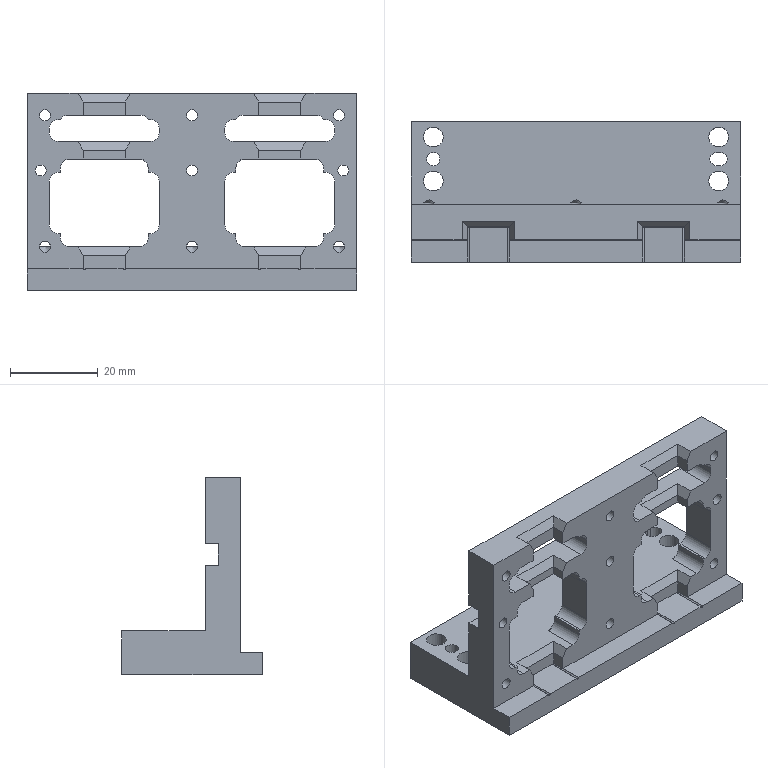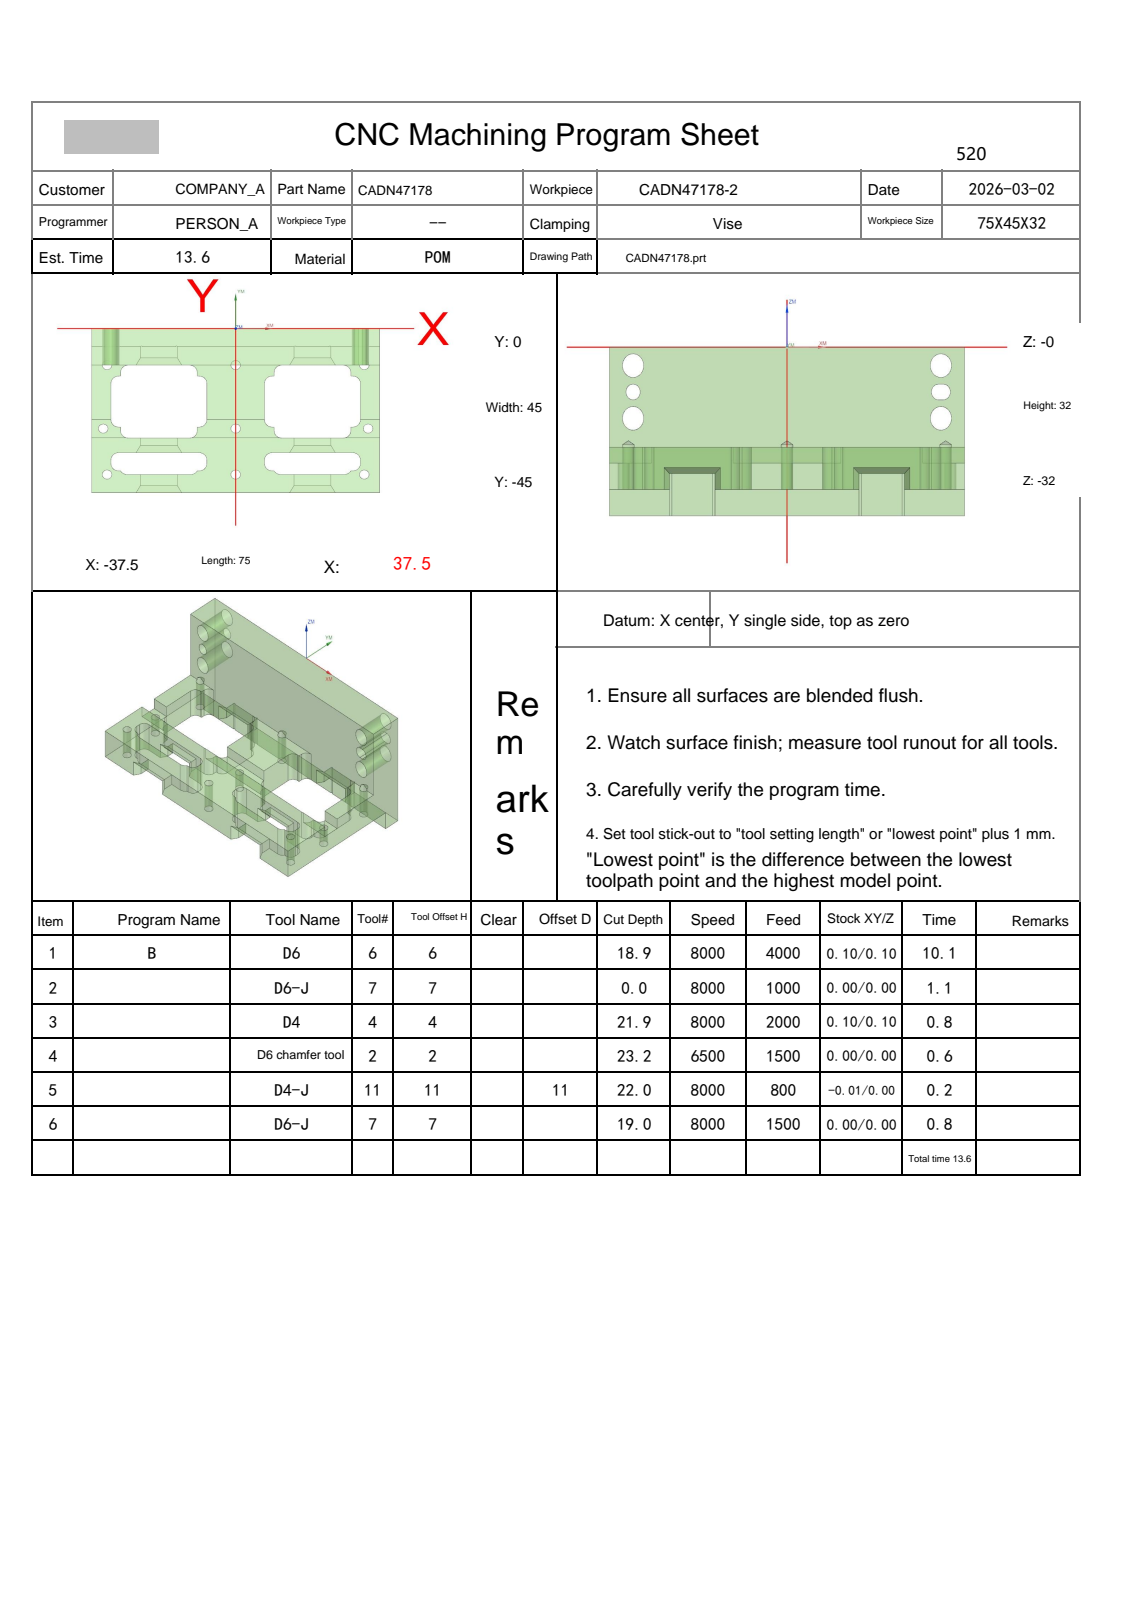NC program | NX | posted by the shop | part box 75 x 32 x 45 mm
Lines 2829 to 3118 of 3118:
N5 T11 M06
(D4-J  D=4. R=0. H=11 ce=-0.01 di=0.00)
G00 G90 G54 X-40.322 Y-27.039 M03 S8000
G43 H11 Z12.5
M08
Z-21.
G01 Z-22. F800.
G41 D11
X-40.29 Y-27.236
G03 X-39.5 Y-27.91 I.79 J.126
G01 X-28.
G03 X-27.206 Y-27.21 I0.0 J.8
G01 G40 X-27.181 Y-27.012
X-27.24 Y-27.37
G41 D11
X-27.36 Y-27.21
G03 X-28. Y-26.89 I-.64 J-.48
G01 X-39.5
G03 X-40.29 Y-27.564 I0.0 J-.8
G01 G40 X-40.322 Y-27.761
Z-21.
G00 Z3.
X-12.819 Y-27.012
Z-21.
G01 Z-22.
G41 D11
X-12.794 Y-27.21
G03 X-12. Y-27.91 I.794 J.1
G01 X12.
G03 X12.794 Y-27.21 I0.0 J.8
G01 G40 X12.819 Y-27.012
X12.76 Y-27.37
G41 D11
X12.64 Y-27.21
G03 X12. Y-26.89 I-.64 J-.48
G01 X-12.
G03 X-12.64 Y-27.21 I0.0 J-.8
G01 G40 X-12.76 Y-27.37
Z-21.
G00 Z3.
X27.181 Y-27.012
Z-21.
G01 Z-22.
G41 D11
X27.206 Y-27.21
G03 X28. Y-27.91 I.794 J.1
G01 X39.5
G03 X40.29 Y-27.236 I0.0 J.8
G01 G40 X40.322 Y-27.039
Y-27.761
G41 D11
X40.29 Y-27.564
G03 X39.5 Y-26.89 I-.79 J-.126
G01 X28.
G03 X27.36 Y-27.21 I0.0 J-.8
G01 G40 X27.24 Y-27.37
Z-21.
G00 Z12.5
G91 G28 Z0.0
M05
M09
G91 G28 Z0.0
M01
N6 T07 M06
(D6-J  D=6. R=0. H=07 ce=0.40 di=0.00)
G00 G90 G54 X1.2 Y-49.2 M03 S7000
G43 H07 Z12.5
M08
Z-17.5
G01 Z-19. F1500.
Y-46.8
G03 X0.0 Y-45.6 I-1.2 J0.0
G01 X-37.502
G02 X-38.1 Y-45.002 I.002 J.6
G01 Y-13.998
G02 X-37.502 Y-13.4 I.6 J-.002
G01 X-34.838
X-34.82 Y-13.396
X-34.818 Y-13.414
X-34.812 Y-13.446
X-34.786 Y-13.466
X-34.754 Y-13.465
G02 X-33.37 Y-14.96 I-.116 J-1.496
G01 Y-14.992
X-33.531 Y-22.602
G02 X-35.03 Y-24.07 I-1.5 J.032
X-36.53 Y-22.57 I0.0 J1.5
G01 Y-22.539
X-36.369 Y-14.929
G02 X-34.896 Y-13.461 I1.5 J-.032
G01 X-34.868 Y-13.46
X-34.862 Y-13.433
X-34.858 Y-13.416
X-34.857 Y-13.397
X-34.838 Y-13.4
X-34.75
X-31.988
X-31.869 Y-13.52
X-31.9 Y-13.6
Y-17.872
Y-23.753
X-26.253 Y-29.4
X-13.747
X-8.1 Y-23.753
Y-13.6
X-8.131 Y-13.52
X-8.012 Y-13.4
X8.012
X8.131 Y-13.52
X8.1 Y-13.6
Y-23.753
X13.747 Y-29.4
X26.253
X31.9 Y-23.753
Y-17.872
Y-13.6
X31.869 Y-13.52
X31.988 Y-13.4
X34.838
X34.855 Y-13.395
X34.857 Y-13.413
X34.864 Y-13.445
X34.891 Y-13.464
X34.923 Y-13.461
G02 X36.369 Y-14.929 I-.053 J-1.499
G01 X36.53 Y-22.539
Y-22.57
G02 X35.03 Y-24.07 I-1.5 J0.0
X33.531 Y-22.602 I0.0 J1.5
G01 X33.37 Y-14.992
Y-14.96
G02 X34.78 Y-13.463 I1.5 J0.0
G01 X34.808 Y-13.462
X34.814 Y-13.434
X34.818 Y-13.416
X34.819 Y-13.397
X34.838 Y-13.4
X37.502
G02 X38.1 Y-13.998 I-.002 J-.6
G01 Y-45.002
G02 X37.502 Y-45.6 I-.6 J.002
G01 X-1.252
G02 X-1.675 Y-45.425 I0.0 J.6
G01 X-4.324 Y-42.775
G03 X-4.748 Y-42.6 I-.424 J-.425
G01 X-34.502
G02 X-35.1 Y-42.002 I.002 J.6
G01 Y-24.25
X-34.98 Y-24.131
X-34.862 Y-24.23
G03 X-34.021 Y-25.874 I2.962 J.478
G01 X-28.374 Y-31.521
G03 X-26.253 Y-32.4 I2.121 J2.121
G01 X-13.747
G03 X-11.626 Y-31.521 I0.0 J3.
G01 X-5.979 Y-25.874
G03 X-5.1 Y-23.753 I-2.121 J2.121
G01 Y-16.998
G02 X-4.502 Y-16.4 I.6 J-.002
G01 X4.502
G02 X5.1 Y-16.998 I-.002 J-.6
G01 Y-23.753
G03 X5.979 Y-25.874 I3. J0.0
G01 X11.626 Y-31.521
G03 X13.747 Y-32.4 I2.121 J2.121
G01 X26.253
G03 X28.374 Y-31.521 I0.0 J3.
G01 X34.021 Y-25.874
G03 X34.862 Y-24.231 I-2.121 J2.121
G01 X34.98 Y-24.131
X35.1 Y-24.25
Y-42.002
G02 X34.502 Y-42.6 I-.6 J.002
G01 X-1.252
G02 X-1.675 Y-42.425 I0.0 J.6
G01 X-4.324 Y-39.776
G03 X-4.748 Y-39.6 I-.424 J-.424
G01 X-31.503
G02 X-32.1 Y-39.003 I.003 J.6
G01 Y-33.484
G02 X-31.5 Y-32.886 I.6 J-.003
X-31.078 Y-33.06 I0.0 J-.6
G01 X-30.495 Y-33.643
G03 X-26.253 Y-35.4 I4.243 J4.243
G01 X-13.747
G03 X-9.504 Y-33.643 I0.0 J6.
G01 X-3.857 Y-27.995
G03 X-2.1 Y-23.753 I-4.243 J4.243
G01 Y-19.997
G02 X-1.503 Y-19.4 I.6 J-.003
G01 X1.503
G02 X2.1 Y-19.997 I-.003 J-.6
G01 Y-23.753
G03 X3.857 Y-27.995 I6. J0.0
G01 X9.505 Y-33.643
G03 X13.747 Y-35.4 I4.243 J4.243
G01 X26.253
G03 X30.495 Y-33.643 I0.0 J6.
G01 X31.078 Y-33.06
G02 X31.5 Y-32.887 I.422 J-.426
X32.1 Y-33.484 I0.0 J-.6
G01 Y-39.003
G02 X31.503 Y-39.6 I-.6 J.003
G01 X-1.252
G02 X-1.675 Y-39.425 I0.0 J.6
G01 X-4.324 Y-36.776
G03 X-4.748 Y-36.6 I-.424 J-.424
G01 X-6.773
G02 X-7.371 Y-36. I.003 J.6
X-7.197 Y-35.578 I.6 J0.0
G01 X-1.736 Y-30.117
G03 X-.505 Y-28.581 I-6.364 J6.364
G02 X0.0 Y-28.305 I.505 J-.324
X.505 Y-28.581 I0.0 J-.6
G03 X1.736 Y-30.117 I7.595 J4.828
G01 X7.197 Y-35.578
G02 X7.371 Y-36. I-.426 J-.422
X6.774 Y-36.6 I-.6 J0.0
G01 X-.98
G02 X-1.34 Y-36.24 I0.0 J.36
G01 X-1.318 Y-36.114
X-.553 Y-34.075
G03 X-.45 Y-33.505 I-1.522 J.57
X-.464 Y-33.288 I-1.625 J0.0
G01 X-.468 Y-33.24
G02 X-.364 Y-32.987 I.36 J0.0
G01 X-.253 Y-32.876
G02 X0.0 Y-32.772 I.253 J-.256
X.253 Y-32.876 I0.0 J-.36
G01 X.364 Y-32.987
G02 X.468 Y-33.24 I-.256 J-.253
X.11 Y-33.6 I-.36 J0.0
G01 X-.11
G02 X-.342 Y-33.513 I.002 J.36
X-.468 Y-33.24 I.235 J.273
X-.364 Y-32.987 I.36 J0.0
G01 X-.253 Y-32.876
G02 X-.027 Y-32.773 I.253 J-.256
G03 X1.082 Y-31.577 I-.091 J1.197
G01 X1.079 Y-31.486
Z-17.5
G00 Z12.5
G00 G90 X38.417 Y-13.995 M03 S8000
Z7.5
Z-3.75
G01 Z-4.75 F1000.
G41 D07
X38.394 Y-13.796
G03 X37.5 Y-13. I-.894 J-.104
G01 X-37.5
G03 X-38.394 Y-13.796 I0.0 J-.9
G01 G40 X-38.417 Y-13.995
Z-3.75
G00 X38.417
Z-8.5
G01 Z-9.5
G41 D07
X38.394 Y-13.796
G03 X37.5 Y-13. I-.894 J-.104
G01 X-37.5
G03 X-38.394 Y-13.796 I0.0 J-.9
G01 G40 X-38.417 Y-13.995
Z-8.5
G00 X38.417
Z-13.25
G01 Z-14.25
G41 D07
X38.394 Y-13.796
G03 X37.5 Y-13. I-.894 J-.104
G01 X-37.5
G03 X-38.394 Y-13.796 I0.0 J-.9
G01 G40 X-38.417 Y-13.995
Z-13.25
G00 X38.417
Z-18.
G01 Z-19.
G41 D07
X38.394 Y-13.796
G03 X37.5 Y-13. I-.894 J-.104
G01 X-37.5
G03 X-38.394 Y-13.796 I0.0 J-.9
G01 G40 X-38.417 Y-13.995
Z-18.
G00 Z7.5
M05
M09
G91 G28 Z0.0
G91 G28 Y0.0
M30
%